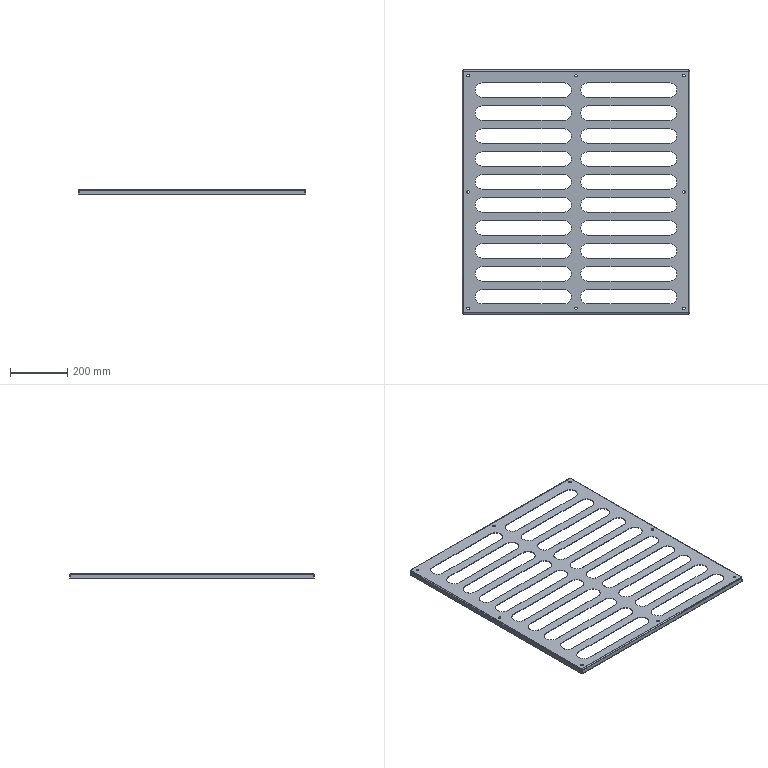Part | SolidWorks | features ICE 3, EdgeFlange 2, LPattern 2, MirrorPattern 2, FlatPattern 1, SMBaseFlange 1, SheetMetal 1 | 1 solid | 186 faces | box 792 x 850 x 20 mm | volume 853821 mm3 | cylinder 92 | plane 78 | spline 16 | commonest cylinder face diameters 50 x60 9 x16 0.4 x4 4 x4 4.4 x4 8 x4